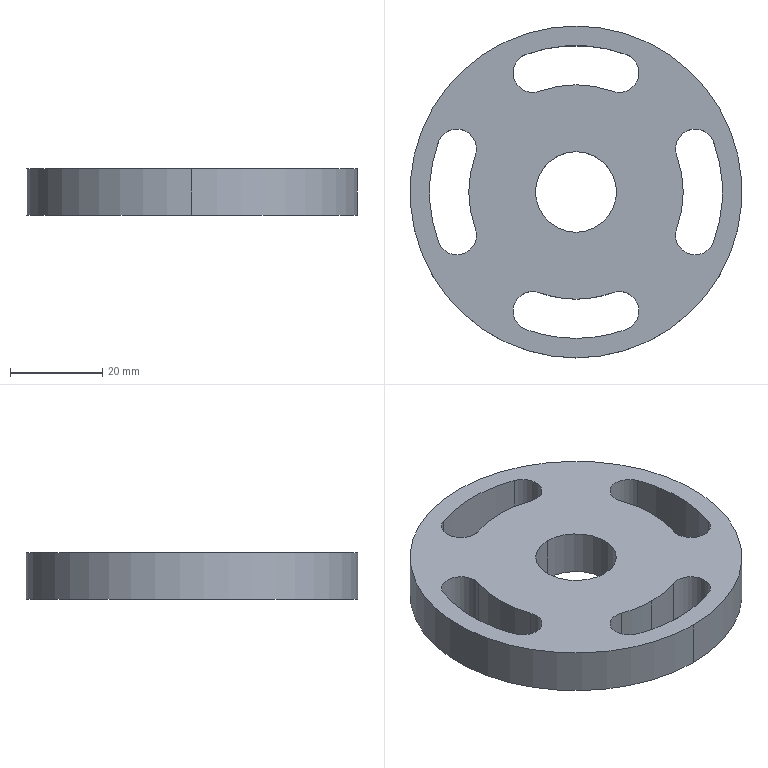NC program | NX | posted with a generic post | part box 72 x 72 x 10 mm
Lines 21188 to 21342 of 21342:
(ZLEVEL_PROFILE_COPY , TOOL : D6JING)
N42374 T08 M6
N42376 G54
N42378 G17 G0 G90 X1.051 Y27.53 S7500 M3
N42380 G43 Z30. H8
N42382 Z-9.5
N42384 G94 G1 Z-11. F1000.
N42386 X0.52 Y28.45
N42388 G3 X0. Y28.75 R0.6
N42390 X-9.833 Y27.016 R28.75
N42392 X-10.58 Y25.414 R1.25
N42394 X-8.978 Y24.667 R1.25
N42396 G2 X8.978 Y24.667 R26.25
N42398 G3 X10.58 Y25.414 R1.25
N42400 X9.833 Y27.016 R1.25
N42402 X0. Y28.75 R28.75
N42404 X-0.52 Y28.45 R0.6
N42406 G1 X-1.051 Y27.53
N42408 Z-9.5
N42410 G0 Z30.
N42412 Y-27.53
N42414 Z-9.5
N42416 G1 Z-11.
N42418 X-0.52 Y-28.45
N42420 G3 X0. Y-28.75 R0.6
N42422 G1 X0.005
N42424 G3 X9.833 Y-27.016 R28.75
N42426 X10.58 Y-25.414 R1.25
N42428 X8.978 Y-24.667 R1.25
N42430 G2 X-8.978 Y-24.667 R26.25
N42432 G3 X-10.58 Y-25.414 R1.25
N42434 X-9.833 Y-27.016 R1.25
N42436 X0. Y-28.75 R28.75
N42438 X0.52 Y-28.45 R0.6
N42440 G1 X1.051 Y-27.53
N42442 Z-9.5
N42444 G0 Z30.
N42446 X-27.53 Y1.051
N42448 Z-9.5
N42450 G1 Z-11.
N42452 X-28.45 Y0.52
N42454 G3 X-28.75 Y0. R0.6
N42456 X-27.016 Y-9.833 R28.75
N42458 X-25.414 Y-10.58 R1.25
N42460 X-24.667 Y-8.978 R1.25
N42462 G2 X-24.667 Y8.978 R26.25
N42464 G3 X-25.414 Y10.58 R1.25
N42466 X-27.016 Y9.833 R1.25
N42468 X-28.75 Y0. R28.75
N42470 X-28.45 Y-0.52 R0.6
N42472 G1 X-27.53 Y-1.051
N42474 Z-9.5
N42476 G0 Z30.
N42478 X27.53
N42480 Z-9.5
N42482 G1 Z-11.
N42484 X28.45 Y-0.52
N42486 G3 X28.75 Y0. R0.6
N42488 X27.016 Y9.833 R28.75
N42490 X25.414 Y10.58 R1.25
N42492 X24.667 Y8.978 R1.25
N42494 G2 X24.667 Y-8.978 R26.25
N42496 G3 X25.414 Y-10.58 R1.25
N42498 X27.016 Y-9.833 R1.25
N42500 X28.75 Y0. R28.75
N42502 X28.45 Y0.52 R0.6
N42504 G1 X27.53 Y1.051
N42506 Z-9.5
N42508 G0 Z30.
N42510 M5
(PLANAR_MILL , TOOL : D6A45)
N42512 T07 M6
N42514 G54
N42516 G17 G0 G90 X1.286 Y29.622 S7500 M3
N42518 G43 Z30. H7
N42520 Z0.5
N42522 G94 G1 Z-1. F1250.
N42524 X0.866 Y30.35
N42526 G3 X0. Y30.85 R1.
N42528 X-10.551 Y28.99 R30.85
N42530 X-12.554 Y24.696 R3.35
N42532 X-8.26 Y22.694 R3.35
N42534 G2 X8.26 Y22.694 R24.15
N42536 G3 X12.554 Y24.696 R3.35
N42538 X10.551 Y28.99 R3.35
N42540 X0. Y30.85 R30.85
N42542 X-0.866 Y30.35 R1.
N42544 G1 X-1.286 Y29.622
N42546 Z0.5
N42548 G0 Z30.
N42550 X-29.622 Y1.286
N42552 Z0.5
N42554 G1 Z-1.
N42556 X-30.35 Y0.866
N42558 G3 X-30.85 Y0. R1.
N42560 X-28.99 Y-10.551 R30.85
N42562 X-24.696 Y-12.554 R3.35
N42564 X-22.694 Y-8.26 R3.35
N42566 G2 X-22.694 Y8.26 R24.15
N42568 G3 X-24.696 Y12.554 R3.35
N42570 X-28.99 Y10.551 R3.35
N42572 X-30.85 Y0. R30.85
N42574 X-30.35 Y-0.866 R1.
N42576 G1 X-29.622 Y-1.286
N42578 Z0.5
N42580 G0 Z30.
N42582 X-1.286 Y-29.622
N42584 Z0.5
N42586 G1 Z-1.
N42588 X-0.866 Y-30.35
N42590 G3 X0. Y-30.85 R1.
N42592 X10.551 Y-28.99 R30.85
N42594 X12.554 Y-24.696 R3.35
N42596 X8.26 Y-22.694 R3.35
N42598 G2 X-8.26 Y-22.694 R24.15
N42600 G3 X-12.554 Y-24.696 R3.35
N42602 X-10.551 Y-28.99 R3.35
N42604 X0. Y-30.85 R30.85
N42606 X0.866 Y-30.35 R1.
N42608 G1 X1.286 Y-29.622
N42610 Z0.5
N42612 G0 Z30.
N42614 X-1.35 Y-6.512
N42616 Z0.5
N42618 G1 Z-1.
N42620 X-0.866 Y-7.35
N42622 G3 X0. Y-7.85 R1.
N42624 X7.85 Y0. R7.85
N42626 X0. Y-7.85 R-7.85
N42628 X0.866 Y-7.35 R1.
N42630 G1 X1.35 Y-6.512
N42632 Z0.5
N42634 G0 Z30.
N42636 X29.622 Y-1.286
N42638 Z0.5
N42640 G1 Z-1.
N42642 X30.35 Y-0.866
N42644 G3 X30.85 Y0. R1.
N42646 X28.99 Y10.551 R30.85
N42648 X24.696 Y12.554 R3.35
N42650 X22.694 Y8.26 R3.35
N42652 G2 X22.694 Y-8.26 R24.15
N42654 G3 X24.696 Y-12.554 R3.35
N42656 X28.99 Y-10.551 R3.35
N42658 X30.85 Y0. R30.85
N42660 X30.35 Y0.866 R1.
N42662 G1 X29.622 Y1.286
N42664 Z0.5
N42666 G0 Z30.
N42668 M5
N42670 M2